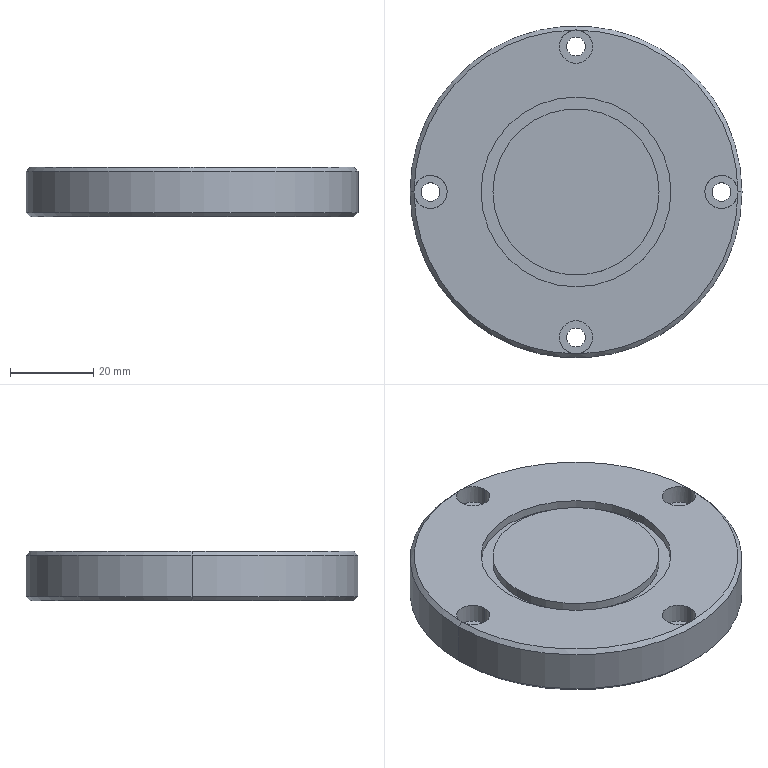Part | STEP file | TJ-DHQM-004-011 | 1 solid | 34 faces | box 79.9 x 79.9 x 12 mm | volume 57718 mm3 | cylinder 22 | plane 8 | cone 4 | commonest cylinder face diameters 4.5 x8 8 x8 40 x2 45.7 x2 79.9 x2
STEP:
#1=CARTESIAN_POINT('',(20.,0.,9.9));
#2=VERTEX_POINT('',#1);
#3=CARTESIAN_POINT('',(-20.,0.,9.9));
#4=VERTEX_POINT('',#3);
#5=CARTESIAN_POINT('',(0.,0.,9.9));
#6=DIRECTION('',(0.,0.,1.));
#7=DIRECTION('',(1.,0.,0.));
#8=AXIS2_PLACEMENT_3D('',#5,#6,#7);
#9=CIRCLE('',#8,20.);
#10=EDGE_CURVE('',#2,#4,#9,.T.);
#11=ORIENTED_EDGE('',*,*,#10,.T.);
#12=CARTESIAN_POINT('',(-20.,0.,12.));
#13=VERTEX_POINT('',#12);
#14=CARTESIAN_POINT('',(-20.,0.,9.9));
#15=DIRECTION('',(0.,0.,1.));
#16=VECTOR('',#15,1000.);
#17=LINE('',#14,#16);
#18=EDGE_CURVE('',#4,#13,#17,.T.);
#19=ORIENTED_EDGE('',*,*,#18,.T.);
#20=CARTESIAN_POINT('',(20.,0.,12.));
#21=VERTEX_POINT('',#20);
#22=CARTESIAN_POINT('',(0.,0.,12.));
#23=DIRECTION('',(0.,0.,1.));
#24=DIRECTION('',(1.,0.,0.));
#25=AXIS2_PLACEMENT_3D('',#22,#23,#24);
#26=CIRCLE('',#25,20.);
#27=EDGE_CURVE('',#21,#13,#26,.T.);
#28=ORIENTED_EDGE('',*,*,#27,.F.);
#29=CARTESIAN_POINT('',(20.,0.,9.9));
#30=DIRECTION('',(0.,0.,1.));
#31=VECTOR('',#30,1000.);
#32=LINE('',#29,#31);
#33=EDGE_CURVE('',#2,#21,#32,.T.);
#34=ORIENTED_EDGE('',*,*,#33,.F.);
#35=EDGE_LOOP('',(#11,#19,#28,#34));
#36=FACE_OUTER_BOUND('',#35,.T.);
#37=CARTESIAN_POINT('',(0.,0.,9.9));
#38=DIRECTION('',(0.,0.,1.));
#39=DIRECTION('',(1.,0.,0.));
#40=AXIS2_PLACEMENT_3D('',#37,#38,#39);
#41=CYLINDRICAL_SURFACE('',#40,20.);
#42=ADVANCED_FACE('',(#36),#41,.T.);
#43=CARTESIAN_POINT('',(-22.85,0.,9.9));
#44=VERTEX_POINT('',#43);
#45=CARTESIAN_POINT('',(22.85,0.,9.9));
#46=VERTEX_POINT('',#45);
#47=CARTESIAN_POINT('',(0.,0.,9.9));
#48=DIRECTION('',(0.,0.,1.));
#49=DIRECTION('',(1.,0.,0.));
#50=AXIS2_PLACEMENT_3D('',#47,#48,#49);
#51=CIRCLE('',#50,22.85);
#52=EDGE_CURVE('',#44,#46,#51,.T.);
#53=ORIENTED_EDGE('',*,*,#52,.F.);
#54=CARTESIAN_POINT('',(-22.85,0.,12.));
#55=VERTEX_POINT('',#54);
#56=CARTESIAN_POINT('',(-22.85,0.,9.9));
#57=DIRECTION('',(0.,0.,1.));
#58=VECTOR('',#57,1000.);
#59=LINE('',#56,#58);
#60=EDGE_CURVE('',#44,#55,#59,.T.);
#61=ORIENTED_EDGE('',*,*,#60,.T.);
#62=CARTESIAN_POINT('',(22.85,0.,12.));
#63=VERTEX_POINT('',#62);
#64=CARTESIAN_POINT('',(0.,0.,12.));
#65=DIRECTION('',(0.,0.,1.));
#66=DIRECTION('',(1.,0.,0.));
#67=AXIS2_PLACEMENT_3D('',#64,#65,#66);
#68=CIRCLE('',#67,22.85);
#69=EDGE_CURVE('',#55,#63,#68,.T.);
#70=ORIENTED_EDGE('',*,*,#69,.T.);
#71=CARTESIAN_POINT('',(22.85,0.,9.9));
#72=DIRECTION('',(0.,0.,1.));
#73=VECTOR('',#72,1000.);
#74=LINE('',#71,#73);
#75=EDGE_CURVE('',#46,#63,#74,.T.);
#76=ORIENTED_EDGE('',*,*,#75,.F.);
#77=EDGE_LOOP('',(#53,#61,#70,#76));
#78=FACE_OUTER_BOUND('',#77,.T.);
#79=CARTESIAN_POINT('',(0.,0.,9.9));
#80=DIRECTION('',(0.,0.,1.));
#81=DIRECTION('',(1.,0.,0.));
#82=AXIS2_PLACEMENT_3D('',#79,#80,#81);
#83=CYLINDRICAL_SURFACE('',#82,22.85);
#84=ADVANCED_FACE('',(#78),#83,.F.);
#85=CARTESIAN_POINT('',(-4.,35.,7.4));
#86=VERTEX_POINT('',#85);
#87=CARTESIAN_POINT('',(4.,35.,7.4));
#88=VERTEX_POINT('',#87);
#89=CARTESIAN_POINT('',(0.,35.,7.4));
#90=DIRECTION('',(0.,0.,1.));
#91=DIRECTION('',(1.,0.,0.));
#92=AXIS2_PLACEMENT_3D('',#89,#90,#91);
#93=CIRCLE('',#92,4.);
#94=EDGE_CURVE('',#86,#88,#93,.T.);
#95=ORIENTED_EDGE('',*,*,#94,.F.);
#96=CARTESIAN_POINT('',(-4.,35.,12.));
#97=VERTEX_POINT('',#96);
#98=CARTESIAN_POINT('',(-4.,35.,12.));
#99=DIRECTION('',(0.,0.,1.));
#100=VECTOR('',#99,1000.);
#101=LINE('',#98,#100);
#102=EDGE_CURVE('',#86,#97,#101,.T.);
#103=ORIENTED_EDGE('',*,*,#102,.T.);
#104=CARTESIAN_POINT('',(4.,35.,12.));
#105=VERTEX_POINT('',#104);
#106=CARTESIAN_POINT('',(0.,35.,12.));
#107=DIRECTION('',(0.,0.,1.));
#108=DIRECTION('',(1.,0.,0.));
#109=AXIS2_PLACEMENT_3D('',#106,#107,#108);
#110=CIRCLE('',#109,4.);
#111=EDGE_CURVE('',#97,#105,#110,.T.);
#112=ORIENTED_EDGE('',*,*,#111,.T.);
#113=CARTESIAN_POINT('',(4.,35.,12.));
#114=DIRECTION('',(0.,0.,1.));
#115=VECTOR('',#114,1000.);
#116=LINE('',#113,#115);
#117=EDGE_CURVE('',#88,#105,#116,.T.);
#118=ORIENTED_EDGE('',*,*,#117,.F.);
#119=EDGE_LOOP('',(#95,#103,#112,#118));
#120=FACE_OUTER_BOUND('',#119,.T.);
#121=CARTESIAN_POINT('',(0.,35.,12.));
#122=DIRECTION('',(0.,0.,1.));
#123=DIRECTION('',(1.,0.,0.));
#124=AXIS2_PLACEMENT_3D('',#121,#122,#123);
#125=CYLINDRICAL_SURFACE('',#124,4.);
#126=ADVANCED_FACE('',(#120),#125,.F.);
#127=CARTESIAN_POINT('',(-2.25,35.,0.));
#128=VERTEX_POINT('',#127);
#129=CARTESIAN_POINT('',(2.25,35.,0.));
#130=VERTEX_POINT('',#129);
#131=CARTESIAN_POINT('',(0.,35.,0.));
#132=DIRECTION('',(0.,0.,1.));
#133=DIRECTION('',(1.,0.,0.));
#134=AXIS2_PLACEMENT_3D('',#131,#132,#133);
#135=CIRCLE('',#134,2.25);
#136=EDGE_CURVE('',#128,#130,#135,.T.);
#137=ORIENTED_EDGE('',*,*,#136,.F.);
#138=CARTESIAN_POINT('',(-2.25,35.,7.4));
#139=VERTEX_POINT('',#138);
#140=CARTESIAN_POINT('',(-2.25,35.,12.));
#141=DIRECTION('',(0.,0.,1.));
#142=VECTOR('',#141,1000.);
#143=LINE('',#140,#142);
#144=EDGE_CURVE('',#128,#139,#143,.T.);
#145=ORIENTED_EDGE('',*,*,#144,.T.);
#146=CARTESIAN_POINT('',(2.25,35.,7.4));
#147=VERTEX_POINT('',#146);
#148=CARTESIAN_POINT('',(0.,35.,7.4));
#149=DIRECTION('',(0.,0.,1.));
#150=DIRECTION('',(1.,0.,0.));
#151=AXIS2_PLACEMENT_3D('',#148,#149,#150);
#152=CIRCLE('',#151,2.25);
#153=EDGE_CURVE('',#139,#147,#152,.T.);
#154=ORIENTED_EDGE('',*,*,#153,.T.);
#155=CARTESIAN_POINT('',(2.25,35.,12.));
#156=DIRECTION('',(0.,0.,1.));
#157=VECTOR('',#156,1000.);
#158=LINE('',#155,#157);
#159=EDGE_CURVE('',#130,#147,#158,.T.);
#160=ORIENTED_EDGE('',*,*,#159,.F.);
#161=EDGE_LOOP('',(#137,#145,#154,#160));
#162=FACE_OUTER_BOUND('',#161,.T.);
#163=CARTESIAN_POINT('',(0.,35.,12.));
#164=DIRECTION('',(0.,0.,1.));
#165=DIRECTION('',(1.,0.,0.));
#166=AXIS2_PLACEMENT_3D('',#163,#164,#165);
#167=CYLINDRICAL_SURFACE('',#166,2.25);
#168=ADVANCED_FACE('',(#162),#167,.F.);
#169=CARTESIAN_POINT('',(-39.,0.,7.4));
#170=VERTEX_POINT('',#169);
#171=CARTESIAN_POINT('',(-31.,0.,7.4));
#172=VERTEX_POINT('',#171);
#173=CARTESIAN_POINT('',(-35.,0.,7.4));
#174=DIRECTION('',(0.,0.,1.));
#175=DIRECTION('',(1.,0.,0.));
#176=AXIS2_PLACEMENT_3D('',#173,#174,#175);
#177=CIRCLE('',#176,4.);
#178=EDGE_CURVE('',#170,#172,#177,.T.);
#179=ORIENTED_EDGE('',*,*,#178,.F.);
#180=CARTESIAN_POINT('',(-39.,0.,11.95));
#181=VERTEX_POINT('',#180);
#182=CARTESIAN_POINT('',(-39.,0.,12.));
#183=DIRECTION('',(0.,0.,1.));
#184=VECTOR('',#183,1000.);
#185=LINE('',#182,#184);
#186=EDGE_CURVE('',#170,#181,#185,.T.);
#187=ORIENTED_EDGE('',*,*,#186,.T.);
#188=CARTESIAN_POINT('',(-38.944,-0.6651,12.));
#189=VERTEX_POINT('',#188);
#190=CARTESIAN_POINT('',(-39.,0.,11.95));
#191=CARTESIAN_POINT('',(-39.,-0.2216,11.95));
#192=CARTESIAN_POINT('',(-38.981,-0.4461,11.967));
#193=CARTESIAN_POINT('',(-38.944,-0.6651,12.));
#194=B_SPLINE_CURVE_WITH_KNOTS('',3,(#190,#191,#192,#193),.UNSPECIFIED.,.F.,.F.,(4,4),(0.0006695,0.001333),.UNSPECIFIED.);
#195=EDGE_CURVE('',#181,#189,#194,.T.);
#196=ORIENTED_EDGE('',*,*,#195,.T.);
#197=CARTESIAN_POINT('',(-31.,0.,12.));
#198=VERTEX_POINT('',#197);
#199=CARTESIAN_POINT('',(-35.,0.,12.));
#200=DIRECTION('',(0.,0.,1.));
#201=DIRECTION('',(1.,0.,0.));
#202=AXIS2_PLACEMENT_3D('',#199,#200,#201);
#203=CIRCLE('',#202,4.);
#204=EDGE_CURVE('',#189,#198,#203,.T.);
#205=ORIENTED_EDGE('',*,*,#204,.T.);
#206=CARTESIAN_POINT('',(-31.,0.,12.));
#207=DIRECTION('',(0.,0.,1.));
#208=VECTOR('',#207,1000.);
#209=LINE('',#206,#208);
#210=EDGE_CURVE('',#172,#198,#209,.T.);
#211=ORIENTED_EDGE('',*,*,#210,.F.);
#212=EDGE_LOOP('',(#179,#187,#196,#205,#211));
#213=FACE_OUTER_BOUND('',#212,.T.);
#214=CARTESIAN_POINT('',(-35.,0.,12.));
#215=DIRECTION('',(0.,0.,1.));
#216=DIRECTION('',(1.,0.,0.));
#217=AXIS2_PLACEMENT_3D('',#214,#215,#216);
#218=CYLINDRICAL_SURFACE('',#217,4.);
#219=ADVANCED_FACE('',(#213),#218,.F.);
#220=CARTESIAN_POINT('',(-37.25,0.,0.));
#221=VERTEX_POINT('',#220);
#222=CARTESIAN_POINT('',(-32.75,0.,0.));
#223=VERTEX_POINT('',#222);
#224=CARTESIAN_POINT('',(-35.,0.,0.));
#225=DIRECTION('',(0.,0.,1.));
#226=DIRECTION('',(1.,0.,0.));
#227=AXIS2_PLACEMENT_3D('',#224,#225,#226);
#228=CIRCLE('',#227,2.25);
#229=EDGE_CURVE('',#221,#223,#228,.T.);
#230=ORIENTED_EDGE('',*,*,#229,.F.);
#231=CARTESIAN_POINT('',(-37.25,0.,7.4));
#232=VERTEX_POINT('',#231);
#233=CARTESIAN_POINT('',(-37.25,0.,12.));
#234=DIRECTION('',(0.,0.,1.));
#235=VECTOR('',#234,1000.);
#236=LINE('',#233,#235);
#237=EDGE_CURVE('',#221,#232,#236,.T.);
#238=ORIENTED_EDGE('',*,*,#237,.T.);
#239=CARTESIAN_POINT('',(-32.75,0.,7.4));
#240=VERTEX_POINT('',#239);
#241=CARTESIAN_POINT('',(-35.,0.,7.4));
#242=DIRECTION('',(0.,0.,1.));
#243=DIRECTION('',(1.,0.,0.));
#244=AXIS2_PLACEMENT_3D('',#241,#242,#243);
#245=CIRCLE('',#244,2.25);
#246=EDGE_CURVE('',#232,#240,#245,.T.);
#247=ORIENTED_EDGE('',*,*,#246,.T.);
#248=CARTESIAN_POINT('',(-32.75,0.,12.));
#249=DIRECTION('',(0.,0.,1.));
#250=VECTOR('',#249,1000.);
#251=LINE('',#248,#250);
#252=EDGE_CURVE('',#223,#240,#251,.T.);
#253=ORIENTED_EDGE('',*,*,#252,.F.);
#254=EDGE_LOOP('',(#230,#238,#247,#253));
#255=FACE_OUTER_BOUND('',#254,.T.);
#256=CARTESIAN_POINT('',(-35.,0.,12.));
#257=DIRECTION('',(0.,0.,1.));
#258=DIRECTION('',(1.,0.,0.));
#259=AXIS2_PLACEMENT_3D('',#256,#257,#258);
#260=CYLINDRICAL_SURFACE('',#259,2.25);
#261=ADVANCED_FACE('',(#255),#260,.F.);
#262=CARTESIAN_POINT('',(-4.,-35.,7.4));
#263=VERTEX_POINT('',#262);
#264=CARTESIAN_POINT('',(4.,-35.,7.4));
#265=VERTEX_POINT('',#264);
#266=CARTESIAN_POINT('',(0.,-35.,7.4));
#267=DIRECTION('',(0.,0.,1.));
#268=DIRECTION('',(1.,0.,0.));
#269=AXIS2_PLACEMENT_3D('',#266,#267,#268);
#270=CIRCLE('',#269,4.);
#271=EDGE_CURVE('',#263,#265,#270,.T.);
#272=ORIENTED_EDGE('',*,*,#271,.F.);
#273=CARTESIAN_POINT('',(-4.,-35.,12.));
#274=VERTEX_POINT('',#273);
#275=CARTESIAN_POINT('',(-4.,-35.,12.));
#276=DIRECTION('',(0.,0.,1.));
#277=VECTOR('',#276,1000.);
#278=LINE('',#275,#277);
#279=EDGE_CURVE('',#263,#274,#278,.T.);
#280=ORIENTED_EDGE('',*,*,#279,.T.);
#281=CARTESIAN_POINT('',(-0.6651,-38.944,12.));
#282=VERTEX_POINT('',#281);
#283=CARTESIAN_POINT('',(0.,-35.,12.));
#284=DIRECTION('',(0.,0.,1.));
#285=DIRECTION('',(1.,0.,0.));
#286=AXIS2_PLACEMENT_3D('',#283,#284,#285);
#287=CIRCLE('',#286,4.);
#288=EDGE_CURVE('',#274,#282,#287,.T.);
#289=ORIENTED_EDGE('',*,*,#288,.T.);
#290=CARTESIAN_POINT('',(0.6651,-38.944,12.));
#291=VERTEX_POINT('',#290);
#292=CARTESIAN_POINT('',(-0.6651,-38.944,12.));
#293=CARTESIAN_POINT('',(-0.4455,-38.981,11.967));
#294=CARTESIAN_POINT('',(-0.2245,-39.,11.95));
#295=CARTESIAN_POINT('',(0.2202,-39.,11.95));
#296=CARTESIAN_POINT('',(0.4454,-38.981,11.967));
#297=CARTESIAN_POINT('',(0.6651,-38.944,12.));
#298=B_SPLINE_CURVE_WITH_KNOTS('',3,(#292,#293,#294,#295,#296,#297),.UNSPECIFIED.,.F.,.F.,(4,2,4),(0.000001333,0.0006674,0.001333),.UNSPECIFIED.);
#299=EDGE_CURVE('',#282,#291,#298,.T.);
#300=ORIENTED_EDGE('',*,*,#299,.T.);
#301=CARTESIAN_POINT('',(4.,-35.,12.));
#302=VERTEX_POINT('',#301);
#303=CARTESIAN_POINT('',(0.,-35.,12.));
#304=DIRECTION('',(0.,0.,1.));
#305=DIRECTION('',(1.,0.,0.));
#306=AXIS2_PLACEMENT_3D('',#303,#304,#305);
#307=CIRCLE('',#306,4.);
#308=EDGE_CURVE('',#291,#302,#307,.T.);
#309=ORIENTED_EDGE('',*,*,#308,.T.);
#310=CARTESIAN_POINT('',(4.,-35.,12.));
#311=DIRECTION('',(0.,0.,1.));
#312=VECTOR('',#311,1000.);
#313=LINE('',#310,#312);
#314=EDGE_CURVE('',#265,#302,#313,.T.);
#315=ORIENTED_EDGE('',*,*,#314,.F.);
#316=EDGE_LOOP('',(#272,#280,#289,#300,#309,#315));
#317=FACE_OUTER_BOUND('',#316,.T.);
#318=CARTESIAN_POINT('',(0.,-35.,12.));
#319=DIRECTION('',(0.,0.,1.));
#320=DIRECTION('',(1.,0.,0.));
#321=AXIS2_PLACEMENT_3D('',#318,#319,#320);
#322=CYLINDRICAL_SURFACE('',#321,4.);
#323=ADVANCED_FACE('',(#317),#322,.F.);
#324=CARTESIAN_POINT('',(-2.25,-35.,0.));
#325=VERTEX_POINT('',#324);
#326=CARTESIAN_POINT('',(2.25,-35.,0.));
#327=VERTEX_POINT('',#326);
#328=CARTESIAN_POINT('',(0.,-35.,0.));
#329=DIRECTION('',(0.,0.,1.));
#330=DIRECTION('',(1.,0.,0.));
#331=AXIS2_PLACEMENT_3D('',#328,#329,#330);
#332=CIRCLE('',#331,2.25);
#333=EDGE_CURVE('',#325,#327,#332,.T.);
#334=ORIENTED_EDGE('',*,*,#333,.F.);
#335=CARTESIAN_POINT('',(-2.25,-35.,7.4));
#336=VERTEX_POINT('',#335);
#337=CARTESIAN_POINT('',(-2.25,-35.,12.));
#338=DIRECTION('',(0.,0.,1.));
#339=VECTOR('',#338,1000.);
#340=LINE('',#337,#339);
#341=EDGE_CURVE('',#325,#336,#340,.T.);
#342=ORIENTED_EDGE('',*,*,#341,.T.);
#343=CARTESIAN_POINT('',(2.25,-35.,7.4));
#344=VERTEX_POINT('',#343);
#345=CARTESIAN_POINT('',(0.,-35.,7.4));
#346=DIRECTION('',(0.,0.,1.));
#347=DIRECTION('',(1.,0.,0.));
#348=AXIS2_PLACEMENT_3D('',#345,#346,#347);
#349=CIRCLE('',#348,2.25);
#350=EDGE_CURVE('',#336,#344,#349,.T.);
#351=ORIENTED_EDGE('',*,*,#350,.T.);
#352=CARTESIAN_POINT('',(2.25,-35.,12.));
#353=DIRECTION('',(0.,0.,1.));
#354=VECTOR('',#353,1000.);
#355=LINE('',#352,#354);
#356=EDGE_CURVE('',#327,#344,#355,.T.);
#357=ORIENTED_EDGE('',*,*,#356,.F.);
#358=EDGE_LOOP('',(#334,#342,#351,#357));
#359=FACE_OUTER_BOUND('',#358,.T.);
#360=CARTESIAN_POINT('',(0.,-35.,12.));
#361=DIRECTION('',(0.,0.,1.));
#362=DIRECTION('',(1.,0.,0.));
#363=AXIS2_PLACEMENT_3D('',#360,#361,#362);
#364=CYLINDRICAL_SURFACE('',#363,2.25);
#365=ADVANCED_FACE('',(#359),#364,.F.);
#366=CARTESIAN_POINT('',(31.,0.,7.4));
#367=VERTEX_POINT('',#366);
#368=CARTESIAN_POINT('',(39.,0.,7.4));
#369=VERTEX_POINT('',#368);
#370=CARTESIAN_POINT('',(35.,0.,7.4));
#371=DIRECTION('',(0.,0.,1.));
#372=DIRECTION('',(1.,0.,0.));
#373=AXIS2_PLACEMENT_3D('',#370,#371,#372);
#374=CIRCLE('',#373,4.);
#375=EDGE_CURVE('',#367,#369,#374,.T.);
#376=ORIENTED_EDGE('',*,*,#375,.F.);
#377=CARTESIAN_POINT('',(31.,0.,12.));
#378=VERTEX_POINT('',#377);
#379=CARTESIAN_POINT('',(31.,0.,12.));
#380=DIRECTION('',(0.,0.,1.));
#381=VECTOR('',#380,1000.);
#382=LINE('',#379,#381);
#383=EDGE_CURVE('',#367,#378,#382,.T.);
#384=ORIENTED_EDGE('',*,*,#383,.T.);
#385=CARTESIAN_POINT('',(38.944,-0.6651,12.));
#386=VERTEX_POINT('',#385);
#387=CARTESIAN_POINT('',(35.,0.,12.));
#388=DIRECTION('',(0.,0.,1.));
#389=DIRECTION('',(1.,0.,0.));
#390=AXIS2_PLACEMENT_3D('',#387,#388,#389);
#391=CIRCLE('',#390,4.);
#392=EDGE_CURVE('',#378,#386,#391,.T.);
#393=ORIENTED_EDGE('',*,*,#392,.T.);
#394=CARTESIAN_POINT('',(39.,0.,11.95));
#395=VERTEX_POINT('',#394);
#396=CARTESIAN_POINT('',(38.944,-0.6651,12.));
#397=CARTESIAN_POINT('',(38.981,-0.4448,11.967));
#398=CARTESIAN_POINT('',(39.,-0.2231,11.95));
#399=CARTESIAN_POINT('',(39.,0.,11.95));
#400=B_SPLINE_CURVE_WITH_KNOTS('',3,(#396,#397,#398,#399),.UNSPECIFIED.,.F.,.F.,(4,4),(0.000001333,0.0006695),.UNSPECIFIED.);
#401=EDGE_CURVE('',#386,#395,#400,.T.);
#402=ORIENTED_EDGE('',*,*,#401,.T.);
#403=CARTESIAN_POINT('',(39.,0.,12.));
#404=DIRECTION('',(0.,0.,1.));
#405=VECTOR('',#404,1000.);
#406=LINE('',#403,#405);
#407=EDGE_CURVE('',#369,#395,#406,.T.);
#408=ORIENTED_EDGE('',*,*,#407,.F.);
#409=EDGE_LOOP('',(#376,#384,#393,#402,#408));
#410=FACE_OUTER_BOUND('',#409,.T.);
#411=CARTESIAN_POINT('',(35.,0.,12.));
#412=DIRECTION('',(0.,0.,1.));
#413=DIRECTION('',(1.,0.,0.));
#414=AXIS2_PLACEMENT_3D('',#411,#412,#413);
#415=CYLINDRICAL_SURFACE('',#414,4.);
#416=ADVANCED_FACE('',(#410),#415,.F.);
#417=CARTESIAN_POINT('',(32.75,0.,0.));
#418=VERTEX_POINT('',#417);
#419=CARTESIAN_POINT('',(37.25,0.,0.));
#420=VERTEX_POINT('',#419);
#421=CARTESIAN_POINT('',(35.,0.,0.));
#422=DIRECTION('',(0.,0.,1.));
#423=DIRECTION('',(1.,0.,0.));
#424=AXIS2_PLACEMENT_3D('',#421,#422,#423);
#425=CIRCLE('',#424,2.25);
#426=EDGE_CURVE('',#418,#420,#425,.T.);
#427=ORIENTED_EDGE('',*,*,#426,.F.);
#428=CARTESIAN_POINT('',(32.75,0.,7.4));
#429=VERTEX_POINT('',#428);
#430=CARTESIAN_POINT('',(32.75,0.,12.));
#431=DIRECTION('',(0.,0.,1.));
#432=VECTOR('',#431,1000.);
#433=LINE('',#430,#432);
#434=EDGE_CURVE('',#418,#429,#433,.T.);
#435=ORIENTED_EDGE('',*,*,#434,.T.);
#436=CARTESIAN_POINT('',(37.25,0.,7.4));
#437=VERTEX_POINT('',#436);
#438=CARTESIAN_POINT('',(35.,0.,7.4));
#439=DIRECTION('',(0.,0.,1.));
#440=DIRECTION('',(1.,0.,0.));
#441=AXIS2_PLACEMENT_3D('',#438,#439,#440);
#442=CIRCLE('',#441,2.25);
#443=EDGE_CURVE('',#429,#437,#442,.T.);
#444=ORIENTED_EDGE('',*,*,#443,.T.);
#445=CARTESIAN_POINT('',(37.25,0.,12.));
#446=DIRECTION('',(0.,0.,1.));
#447=VECTOR('',#446,1000.);
#448=LINE('',#445,#447);
#449=EDGE_CURVE('',#420,#437,#448,.T.);
#450=ORIENTED_EDGE('',*,*,#449,.F.);
#451=EDGE_LOOP('',(#427,#435,#444,#450));
#452=FACE_OUTER_BOUND('',#451,.T.);
#453=CARTESIAN_POINT('',(35.,0.,12.));
#454=DIRECTION('',(0.,0.,1.));
#455=DIRECTION('',(1.,0.,0.));
#456=AXIS2_PLACEMENT_3D('',#453,#454,#455);
#457=CYLINDRICAL_SURFACE('',#456,2.25);
#458=ADVANCED_FACE('',(#452),#457,.F.);
#459=CARTESIAN_POINT('',(38.944,0.6651,12.));
#460=VERTEX_POINT('',#459);
#461=CARTESIAN_POINT('',(39.,0.,11.95));
#462=CARTESIAN_POINT('',(39.,0.2216,11.95));
#463=CARTESIAN_POINT('',(38.981,0.4461,11.967));
#464=CARTESIAN_POINT('',(38.944,0.6651,12.));
#465=B_SPLINE_CURVE_WITH_KNOTS('',3,(#461,#462,#463,#464),.UNSPECIFIED.,.F.,.F.,(4,4),(0.0006695,0.001333),.UNSPECIFIED.);
#466=EDGE_CURVE('',#395,#460,#465,.T.);
#467=ORIENTED_EDGE('',*,*,#466,.F.);
#468=CARTESIAN_POINT('',(39.95,0.,11.));
#469=VERTEX_POINT('',#468);
#470=CARTESIAN_POINT('',(38.95,0.,12.));
#471=DIRECTION('',(0.7071,0.,-0.7071));
#472=VECTOR('',#471,1000.);
#473=LINE('',#470,#472);
#474=EDGE_CURVE('',#395,#469,#473,.T.);
#475=ORIENTED_EDGE('',*,*,#474,.T.);
#476=CARTESIAN_POINT('',(-39.95,0.,11.));
#477=VERTEX_POINT('',#476);
#478=CARTESIAN_POINT('',(0.,0.,11.));
#479=DIRECTION('',(0.,0.,-1.));
#480=DIRECTION('',(1.,0.,0.));
#481=AXIS2_PLACEMENT_3D('',#478,#479,#480);
#482=CIRCLE('',#481,39.95);
#483=EDGE_CURVE('',#477,#469,#482,.T.);
#484=ORIENTED_EDGE('',*,*,#483,.F.);
#485=CARTESIAN_POINT('',(-38.95,0.,12.));
#486=DIRECTION('',(-0.7071,0.,-0.7071));
#487=VECTOR('',#486,1000.);
#488=LINE('',#485,#487);
#489=EDGE_CURVE('',#181,#477,#488,.T.);
#490=ORIENTED_EDGE('',*,*,#489,.F.);
#491=CARTESIAN_POINT('',(-38.944,0.6651,12.));
#492=VERTEX_POINT('',#491);
#493=CARTESIAN_POINT('',(-38.944,0.6651,12.));
#494=CARTESIAN_POINT('',(-38.981,0.4448,11.967));
#495=CARTESIAN_POINT('',(-39.,0.2231,11.95));
#496=CARTESIAN_POINT('',(-39.,0.,11.95));
#497=B_SPLINE_CURVE_WITH_KNOTS('',3,(#493,#494,#495,#496),.UNSPECIFIED.,.F.,.F.,(4,4),(0.000001333,0.0006695),.UNSPECIFIED.);
#498=EDGE_CURVE('',#492,#181,#497,.T.);
#499=ORIENTED_EDGE('',*,*,#498,.F.);
#500=CARTESIAN_POINT('',(-0.6651,38.944,12.));
#501=VERTEX_POINT('',#500);
#502=CARTESIAN_POINT('',(0.,0.,12.));
#503=DIRECTION('',(0.,0.,1.));
#504=DIRECTION('',(1.,0.,0.));
#505=AXIS2_PLACEMENT_3D('',#502,#503,#504);
#506=CIRCLE('',#505,38.95);
#507=EDGE_CURVE('',#501,#492,#506,.T.);
#508=ORIENTED_EDGE('',*,*,#507,.F.);
#509=CARTESIAN_POINT('',(0.6651,38.944,12.));
#510=VERTEX_POINT('',#509);
#511=CARTESIAN_POINT('',(0.6651,38.944,12.));
#512=CARTESIAN_POINT('',(0.4455,38.981,11.967));
#513=CARTESIAN_POINT('',(0.2245,39.,11.95));
#514=CARTESIAN_POINT('',(-0.2202,39.,11.95));
#515=CARTESIAN_POINT('',(-0.4454,38.981,11.967));
#516=CARTESIAN_POINT('',(-0.6651,38.944,12.));
#517=B_SPLINE_CURVE_WITH_KNOTS('',3,(#511,#512,#513,#514,#515,#516),.UNSPECIFIED.,.F.,.F.,(4,2,4),(0.000001333,0.0006674,0.001333),.UNSPECIFIED.);
#518=EDGE_CURVE('',#510,#501,#517,.T.);
#519=ORIENTED_EDGE('',*,*,#518,.F.);
#520=CARTESIAN_POINT('',(0.,0.,12.));
#521=DIRECTION('',(0.,0.,1.));
#522=DIRECTION('',(1.,0.,0.));
#523=AXIS2_PLACEMENT_3D('',#520,#521,#522);
#524=CIRCLE('',#523,38.95);
#525=EDGE_CURVE('',#460,#510,#524,.T.);
#526=ORIENTED_EDGE('',*,*,#525,.F.);
#527=EDGE_LOOP('',(#467,#475,#484,#490,#499,#508,#519,#526));
#528=FACE_OUTER_BOUND('',#527,.T.);
#529=CARTESIAN_POINT('',(0.,0.,12.));
#530=DIRECTION('',(0.,0.,-1.));
#531=DIRECTION('',(-1.,0.,0.));
#532=AXIS2_PLACEMENT_3D('',#529,#530,#531);
#533=CONICAL_SURFACE('',#532,38.95,0.7854);
#534=ADVANCED_FACE('',(#528),#533,.T.);
#535=CARTESIAN_POINT('',(-38.95,0.,0.));
#536=VERTEX_POINT('',#535);
#537=CARTESIAN_POINT('',(38.95,0.,0.));
#538=VERTEX_POINT('',#537);
#539=CARTESIAN_POINT('',(0.,0.,0.));
#540=DIRECTION('',(0.,0.,-1.));
#541=DIRECTION('',(1.,0.,0.));
#542=AXIS2_PLACEMENT_3D('',#539,#540,#541);
#543=CIRCLE('',#542,38.95);
#544=EDGE_CURVE('',#536,#538,#543,.T.);
#545=ORIENTED_EDGE('',*,*,#544,.F.);
#546=CARTESIAN_POINT('',(-39.95,0.,1.));
#547=VERTEX_POINT('',#546);
#548=CARTESIAN_POINT('',(-39.95,0.,1.));
#549=DIRECTION('',(-0.7071,0.,0.7071));
#550=VECTOR('',#549,1000.);
#551=LINE('',#548,#550);
#552=EDGE_CURVE('',#536,#547,#551,.T.);
#553=ORIENTED_EDGE('',*,*,#552,.T.);
#554=CARTESIAN_POINT('',(39.95,0.,1.));
#555=VERTEX_POINT('',#554);
#556=CARTESIAN_POINT('',(0.,0.,1.));
#557=DIRECTION('',(0.,0.,1.));
#558=DIRECTION('',(1.,0.,0.));
#559=AXIS2_PLACEMENT_3D('',#556,#557,#558);
#560=CIRCLE('',#559,39.95);
#561=EDGE_CURVE('',#555,#547,#560,.T.);
#562=ORIENTED_EDGE('',*,*,#561,.F.);
#563=CARTESIAN_POINT('',(39.95,0.,1.));
#564=DIRECTION('',(0.7071,0.,0.7071));
#565=VECTOR('',#564,1000.);
#566=LINE('',#563,#565);
#567=EDGE_CURVE('',#538,#555,#566,.T.);
#568=ORIENTED_EDGE('',*,*,#567,.F.);
#569=EDGE_LOOP('',(#545,#553,#562,#568));
#570=FACE_OUTER_BOUND('',#569,.T.);
#571=CARTESIAN_POINT('',(0.,0.,1.));
#572=DIRECTION('',(0.,0.,1.));
#573=DIRECTION('',(1.,0.,0.));
#574=AXIS2_PLACEMENT_3D('',#571,#572,#573);
#575=CONICAL_SURFACE('',#574,39.95,0.7854);
#576=ADVANCED_FACE('',(#570),#575,.T.);
#577=ORIENTED_EDGE('',*,*,#483,.T.);
#578=CARTESIAN_POINT('',(39.95,0.,12.));
#579=DIRECTION('',(0.,0.,-1.));
#580=VECTOR('',#579,1000.);
#581=LINE('',#578,#580);
#582=EDGE_CURVE('',#469,#555,#581,.T.);
#583=ORIENTED_EDGE('',*,*,#582,.T.);
#584=ORIENTED_EDGE('',*,*,#561,.T.);
#585=CARTESIAN_POINT('',(-39.95,0.,12.));
#586=DIRECTION('',(0.,0.,-1.));
#587=VECTOR('',#586,1000.);
#588=LINE('',#585,#587);
#589=EDGE_CURVE('',#477,#547,#588,.T.);
#590=ORIENTED_EDGE('',*,*,#589,.F.);
#591=EDGE_LOOP('',(#577,#583,#584,#590));
#592=FACE_OUTER_BOUND('',#591,.T.);
#593=CARTESIAN_POINT('',(0.,0.,12.));
#594=DIRECTION('',(0.,0.,-1.));
#595=DIRECTION('',(-1.,0.,0.));
#596=AXIS2_PLACEMENT_3D('',#593,#594,#595);
#597=CYLINDRICAL_SURFACE('',#596,39.95);
#598=ADVANCED_FACE('',(#592),#597,.T.);
#599=ORIENTED_EDGE('',*,*,#582,.F.);
#600=CARTESIAN_POINT('',(0.,0.,11.));
#601=DIRECTION('',(0.,0.,-1.));
#602=DIRECTION('',(1.,0.,0.));
#603=AXIS2_PLACEMENT_3D('',#600,#601,#602);
#604=CIRCLE('',#603,39.95);
#605=EDGE_CURVE('',#469,#477,#604,.T.);
#606=ORIENTED_EDGE('',*,*,#605,.T.);
#607=ORIENTED_EDGE('',*,*,#589,.T.);
#608=CARTESIAN_POINT('',(0.,0.,1.));
#609=DIRECTION('',(0.,0.,1.));
#610=DIRECTION('',(1.,0.,0.));
#611=AXIS2_PLACEMENT_3D('',#608,#609,#610);
#612=CIRCLE('',#611,39.95);
#613=EDGE_CURVE('',#547,#555,#612,.T.);
#614=ORIENTED_EDGE('',*,*,#613,.T.);
#615=EDGE_LOOP('',(#599,#606,#607,#614));
#616=FACE_OUTER_BOUND('',#615,.T.);
#617=CARTESIAN_POINT('',(0.,0.,12.));
#618=DIRECTION('',(0.,0.,-1.));
#619=DIRECTION('',(-1.,0.,0.));
#620=AXIS2_PLACEMENT_3D('',#617,#618,#619);
#621=CYLINDRICAL_SURFACE('',#620,39.95);
#622=ADVANCED_FACE('',(#616),#621,.T.);
#623=CARTESIAN_POINT('',(0.,0.,12.));
#624=DIRECTION('',(0.,0.,1.));
#625=DIRECTION('',(1.,0.,0.));
#626=AXIS2_PLACEMENT_3D('',#623,#624,#625);
#627=CIRCLE('',#626,22.85);
#628=EDGE_CURVE('',#63,#55,#627,.T.);
#629=ORIENTED_EDGE('',*,*,#628,.F.);
#630=ORIENTED_EDGE('',*,*,#69,.F.);
#631=EDGE_LOOP('',(#629,#630));
#632=FACE_BOUND('',#631,.T.);
#633=CARTESIAN_POINT('',(0.,35.,12.));
#634=DIRECTION('',(0.,0.,1.));
#635=DIRECTION('',(1.,0.,0.));
#636=AXIS2_PLACEMENT_3D('',#633,#634,#635);
#637=CIRCLE('',#636,4.);
#638=EDGE_CURVE('',#501,#97,#637,.T.);
#639=ORIENTED_EDGE('',*,*,#638,.F.);
#640=ORIENTED_EDGE('',*,*,#507,.T.);
#641=CARTESIAN_POINT('',(-35.,0.,12.));
#642=DIRECTION('',(0.,0.,1.));
#643=DIRECTION('',(1.,0.,0.));
#644=AXIS2_PLACEMENT_3D('',#641,#642,#643);
#645=CIRCLE('',#644,4.);
#646=EDGE_CURVE('',#198,#492,#645,.T.);
#647=ORIENTED_EDGE('',*,*,#646,.F.);
#648=ORIENTED_EDGE('',*,*,#204,.F.);
#649=CARTESIAN_POINT('',(0.,0.,12.));
#650=DIRECTION('',(0.,0.,1.));
#651=DIRECTION('',(1.,0.,0.));
#652=AXIS2_PLACEMENT_3D('',#649,#650,#651);
#653=CIRCLE('',#652,38.95);
#654=EDGE_CURVE('',#189,#282,#653,.T.);
#655=ORIENTED_EDGE('',*,*,#654,.T.);
#656=ORIENTED_EDGE('',*,*,#288,.F.);
#657=CARTESIAN_POINT('',(0.,-35.,12.));
#658=DIRECTION('',(0.,0.,1.));
#659=DIRECTION('',(1.,0.,0.));
#660=AXIS2_PLACEMENT_3D('',#657,#658,#659);
#661=CIRCLE('',#660,4.);
#662=EDGE_CURVE('',#302,#274,#661,.T.);
#663=ORIENTED_EDGE('',*,*,#662,.F.);
#664=ORIENTED_EDGE('',*,*,#308,.F.);
#665=CARTESIAN_POINT('',(0.,0.,12.));
#666=DIRECTION('',(0.,0.,1.));
#667=DIRECTION('',(1.,0.,0.));
#668=AXIS2_PLACEMENT_3D('',#665,#666,#667);
#669=CIRCLE('',#668,38.95);
#670=EDGE_CURVE('',#291,#386,#669,.T.);
#671=ORIENTED_EDGE('',*,*,#670,.T.);
#672=ORIENTED_EDGE('',*,*,#392,.F.);
#673=CARTESIAN_POINT('',(35.,0.,12.));
#674=DIRECTION('',(0.,0.,1.));
#675=DIRECTION('',(1.,0.,0.));
#676=AXIS2_PLACEMENT_3D('',#673,#674,#675);
#677=CIRCLE('',#676,4.);
#678=EDGE_CURVE('',#460,#378,#677,.T.);
#679=ORIENTED_EDGE('',*,*,#678,.F.);
#680=ORIENTED_EDGE('',*,*,#525,.T.);
#681=CARTESIAN_POINT('',(0.,35.,12.));
#682=DIRECTION('',(0.,0.,1.));
#683=DIRECTION('',(1.,0.,0.));
#684=AXIS2_PLACEMENT_3D('',#681,#682,#683);
#685=CIRCLE('',#684,4.);
#686=EDGE_CURVE('',#105,#510,#685,.T.);
#687=ORIENTED_EDGE('',*,*,#686,.F.);
#688=ORIENTED_EDGE('',*,*,#111,.F.);
#689=EDGE_LOOP('',(#639,#640,#647,#648,#655,#656,#663,#664,#671,#672,#679,#680,#687,#688));
#690=FACE_OUTER_BOUND('',#689,.T.);
#691=CARTESIAN_POINT('',(0.,0.,12.));
#692=DIRECTION('',(0.,0.,1.));
#693=DIRECTION('',(1.,0.,0.));
#694=AXIS2_PLACEMENT_3D('',#691,#692,#693);
#695=PLANE('',#694);
#696=ADVANCED_FACE('',(#632,#690),#695,.T.);
#697=CARTESIAN_POINT('',(0.,35.,0.));
#698=DIRECTION('',(0.,0.,1.));
#699=DIRECTION('',(1.,0.,0.));
#700=AXIS2_PLACEMENT_3D('',#697,#698,#699);
#701=CIRCLE('',#700,2.25);
#702=EDGE_CURVE('',#130,#128,#701,.T.);
#703=ORIENTED_EDGE('',*,*,#702,.T.);
#704=ORIENTED_EDGE('',*,*,#136,.T.);
#705=EDGE_LOOP('',(#703,#704));
#706=FACE_BOUND('',#705,.T.);
#707=CARTESIAN_POINT('',(-35.,0.,0.));
#708=DIRECTION('',(0.,0.,1.));
#709=DIRECTION('',(1.,0.,0.));
#710=AXIS2_PLACEMENT_3D('',#707,#708,#709);
#711=CIRCLE('',#710,2.25);
#712=EDGE_CURVE('',#223,#221,#711,.T.);
#713=ORIENTED_EDGE('',*,*,#712,.T.);
#714=ORIENTED_EDGE('',*,*,#229,.T.);
#715=EDGE_LOOP('',(#713,#714));
#716=FACE_BOUND('',#715,.T.);
#717=CARTESIAN_POINT('',(0.,-35.,0.));
#718=DIRECTION('',(0.,0.,1.));
#719=DIRECTION('',(1.,0.,0.));
#720=AXIS2_PLACEMENT_3D('',#717,#718,#719);
#721=CIRCLE('',#720,2.25);
#722=EDGE_CURVE('',#327,#325,#721,.T.);
#723=ORIENTED_EDGE('',*,*,#722,.T.);
#724=ORIENTED_EDGE('',*,*,#333,.T.);
#725=EDGE_LOOP('',(#723,#724));
#726=FACE_BOUND('',#725,.T.);
#727=CARTESIAN_POINT('',(35.,0.,0.));
#728=DIRECTION('',(0.,0.,1.));
#729=DIRECTION('',(1.,0.,0.));
#730=AXIS2_PLACEMENT_3D('',#727,#728,#729);
#731=CIRCLE('',#730,2.25);
#732=EDGE_CURVE('',#420,#418,#731,.T.);
#733=ORIENTED_EDGE('',*,*,#732,.T.);
#734=ORIENTED_EDGE('',*,*,#426,.T.);
#735=EDGE_LOOP('',(#733,#734));
#736=FACE_BOUND('',#735,.T.);
#737=CARTESIAN_POINT('',(0.,0.,0.));
#738=DIRECTION('',(0.,0.,-1.));
#739=DIRECTION('',(1.,0.,0.));
#740=AXIS2_PLACEMENT_3D('',#737,#738,#739);
#741=CIRCLE('',#740,38.95);
#742=EDGE_CURVE('',#538,#536,#741,.T.);
#743=ORIENTED_EDGE('',*,*,#742,.T.);
#744=ORIENTED_EDGE('',*,*,#544,.T.);
#745=EDGE_LOOP('',(#743,#744));
#746=FACE_OUTER_BOUND('',#745,.T.);
#747=CARTESIAN_POINT('',(0.,0.,0.));
#748=DIRECTION('',(0.,0.,1.));
#749=DIRECTION('',(1.,0.,0.));
#750=AXIS2_PLACEMENT_3D('',#747,#748,#749);
#751=PLANE('',#750);
#752=ADVANCED_FACE('',(#706,#716,#726,#736,#746),#751,.F.);
#753=ORIENTED_EDGE('',*,*,#552,.F.);
#754=ORIENTED_EDGE('',*,*,#742,.F.);
#755=ORIENTED_EDGE('',*,*,#567,.T.);
#756=ORIENTED_EDGE('',*,*,#613,.F.);
#757=EDGE_LOOP('',(#753,#754,#755,#756));
#758=FACE_OUTER_BOUND('',#757,.T.);
#759=CARTESIAN_POINT('',(0.,0.,1.));
#760=DIRECTION('',(0.,0.,1.));
#761=DIRECTION('',(1.,0.,0.));
#762=AXIS2_PLACEMENT_3D('',#759,#760,#761);
#763=CONICAL_SURFACE('',#762,39.95,0.7854);
#764=ADVANCED_FACE('',(#758),#763,.T.);
#765=ORIENTED_EDGE('',*,*,#474,.F.);
#766=ORIENTED_EDGE('',*,*,#401,.F.);
#767=ORIENTED_EDGE('',*,*,#670,.F.);
#768=ORIENTED_EDGE('',*,*,#299,.F.);
#769=ORIENTED_EDGE('',*,*,#654,.F.);
#770=ORIENTED_EDGE('',*,*,#195,.F.);
#771=ORIENTED_EDGE('',*,*,#489,.T.);
#772=ORIENTED_EDGE('',*,*,#605,.F.);
#773=EDGE_LOOP('',(#765,#766,#767,#768,#769,#770,#771,#772));
#774=FACE_OUTER_BOUND('',#773,.T.);
#775=CARTESIAN_POINT('',(0.,0.,12.));
#776=DIRECTION('',(0.,0.,-1.));
#777=DIRECTION('',(-1.,0.,0.));
#778=AXIS2_PLACEMENT_3D('',#775,#776,#777);
#779=CONICAL_SURFACE('',#778,38.95,0.7854);
#780=ADVANCED_FACE('',(#774),#779,.T.);
#781=ORIENTED_EDGE('',*,*,#434,.F.);
#782=ORIENTED_EDGE('',*,*,#732,.F.);
#783=ORIENTED_EDGE('',*,*,#449,.T.);
#784=CARTESIAN_POINT('',(35.,0.,7.4));
#785=DIRECTION('',(0.,0.,1.));
#786=DIRECTION('',(1.,0.,0.));
#787=AXIS2_PLACEMENT_3D('',#784,#785,#786);
#788=CIRCLE('',#787,2.25);
#789=EDGE_CURVE('',#437,#429,#788,.T.);
#790=ORIENTED_EDGE('',*,*,#789,.T.);
#791=EDGE_LOOP('',(#781,#782,#783,#790));
#792=FACE_OUTER_BOUND('',#791,.T.);
#793=CARTESIAN_POINT('',(35.,0.,12.));
#794=DIRECTION('',(0.,0.,1.));
#795=DIRECTION('',(1.,0.,0.));
#796=AXIS2_PLACEMENT_3D('',#793,#794,#795);
#797=CYLINDRICAL_SURFACE('',#796,2.25);
#798=ADVANCED_FACE('',(#792),#797,.F.);
#799=ORIENTED_EDGE('',*,*,#789,.F.);
#800=ORIENTED_EDGE('',*,*,#443,.F.);
#801=EDGE_LOOP('',(#799,#800));
#802=FACE_BOUND('',#801,.T.);
#803=CARTESIAN_POINT('',(35.,0.,7.4));
#804=DIRECTION('',(0.,0.,1.));
#805=DIRECTION('',(1.,0.,0.));
#806=AXIS2_PLACEMENT_3D('',#803,#804,#805);
#807=CIRCLE('',#806,4.);
#808=EDGE_CURVE('',#369,#367,#807,.T.);
#809=ORIENTED_EDGE('',*,*,#808,.T.);
#810=ORIENTED_EDGE('',*,*,#375,.T.);
#811=EDGE_LOOP('',(#809,#810));
#812=FACE_OUTER_BOUND('',#811,.T.);
#813=CARTESIAN_POINT('',(37.25,0.,7.4));
#814=DIRECTION('',(0.,0.,-1.));
#815=DIRECTION('',(-1.,0.,0.));
#816=AXIS2_PLACEMENT_3D('',#813,#814,#815);
#817=PLANE('',#816);
#818=ADVANCED_FACE('',(#802,#812),#817,.F.);
#819=ORIENTED_EDGE('',*,*,#383,.F.);
#820=ORIENTED_EDGE('',*,*,#808,.F.);
#821=ORIENTED_EDGE('',*,*,#407,.T.);
#822=ORIENTED_EDGE('',*,*,#466,.T.);
#823=ORIENTED_EDGE('',*,*,#678,.T.);
#824=EDGE_LOOP('',(#819,#820,#821,#822,#823));
#825=FACE_OUTER_BOUND('',#824,.T.);
#826=CARTESIAN_POINT('',(35.,0.,12.));
#827=DIRECTION('',(0.,0.,1.));
#828=DIRECTION('',(1.,0.,0.));
#829=AXIS2_PLACEMENT_3D('',#826,#827,#828);
#830=CYLINDRICAL_SURFACE('',#829,4.);
#831=ADVANCED_FACE('',(#825),#830,.F.);
#832=ORIENTED_EDGE('',*,*,#341,.F.);
#833=ORIENTED_EDGE('',*,*,#722,.F.);
#834=ORIENTED_EDGE('',*,*,#356,.T.);
#835=CARTESIAN_POINT('',(0.,-35.,7.4));
#836=DIRECTION('',(0.,0.,1.));
#837=DIRECTION('',(1.,0.,0.));
#838=AXIS2_PLACEMENT_3D('',#835,#836,#837);
#839=CIRCLE('',#838,2.25);
#840=EDGE_CURVE('',#344,#336,#839,.T.);
#841=ORIENTED_EDGE('',*,*,#840,.T.);
#842=EDGE_LOOP('',(#832,#833,#834,#841));
#843=FACE_OUTER_BOUND('',#842,.T.);
#844=CARTESIAN_POINT('',(0.,-35.,12.));
#845=DIRECTION('',(0.,0.,1.));
#846=DIRECTION('',(1.,0.,0.));
#847=AXIS2_PLACEMENT_3D('',#844,#845,#846);
#848=CYLINDRICAL_SURFACE('',#847,2.25);
#849=ADVANCED_FACE('',(#843),#848,.F.);
#850=ORIENTED_EDGE('',*,*,#840,.F.);
#851=ORIENTED_EDGE('',*,*,#350,.F.);
#852=EDGE_LOOP('',(#850,#851));
#853=FACE_BOUND('',#852,.T.);
#854=CARTESIAN_POINT('',(0.,-35.,7.4));
#855=DIRECTION('',(0.,0.,1.));
#856=DIRECTION('',(1.,0.,0.));
#857=AXIS2_PLACEMENT_3D('',#854,#855,#856);
#858=CIRCLE('',#857,4.);
#859=EDGE_CURVE('',#265,#263,#858,.T.);
#860=ORIENTED_EDGE('',*,*,#859,.T.);
#861=ORIENTED_EDGE('',*,*,#271,.T.);
#862=EDGE_LOOP('',(#860,#861));
#863=FACE_OUTER_BOUND('',#862,.T.);
#864=CARTESIAN_POINT('',(2.25,-35.,7.4));
#865=DIRECTION('',(0.,0.,-1.));
#866=DIRECTION('',(-1.,0.,0.));
#867=AXIS2_PLACEMENT_3D('',#864,#865,#866);
#868=PLANE('',#867);
#869=ADVANCED_FACE('',(#853,#863),#868,.F.);
#870=ORIENTED_EDGE('',*,*,#279,.F.);
#871=ORIENTED_EDGE('',*,*,#859,.F.);
#872=ORIENTED_EDGE('',*,*,#314,.T.);
#873=ORIENTED_EDGE('',*,*,#662,.T.);
#874=EDGE_LOOP('',(#870,#871,#872,#873));
#875=FACE_OUTER_BOUND('',#874,.T.);
#876=CARTESIAN_POINT('',(0.,-35.,12.));
#877=DIRECTION('',(0.,0.,1.));
#878=DIRECTION('',(1.,0.,0.));
#879=AXIS2_PLACEMENT_3D('',#876,#877,#878);
#880=CYLINDRICAL_SURFACE('',#879,4.);
#881=ADVANCED_FACE('',(#875),#880,.F.);
#882=ORIENTED_EDGE('',*,*,#237,.F.);
#883=ORIENTED_EDGE('',*,*,#712,.F.);
#884=ORIENTED_EDGE('',*,*,#252,.T.);
#885=CARTESIAN_POINT('',(-35.,0.,7.4));
#886=DIRECTION('',(0.,0.,1.));
#887=DIRECTION('',(1.,0.,0.));
#888=AXIS2_PLACEMENT_3D('',#885,#886,#887);
#889=CIRCLE('',#888,2.25);
#890=EDGE_CURVE('',#240,#232,#889,.T.);
#891=ORIENTED_EDGE('',*,*,#890,.T.);
#892=EDGE_LOOP('',(#882,#883,#884,#891));
#893=FACE_OUTER_BOUND('',#892,.T.);
#894=CARTESIAN_POINT('',(-35.,0.,12.));
#895=DIRECTION('',(0.,0.,1.));
#896=DIRECTION('',(1.,0.,0.));
#897=AXIS2_PLACEMENT_3D('',#894,#895,#896);
#898=CYLINDRICAL_SURFACE('',#897,2.25);
#899=ADVANCED_FACE('',(#893),#898,.F.);
#900=ORIENTED_EDGE('',*,*,#890,.F.);
#901=ORIENTED_EDGE('',*,*,#246,.F.);
#902=EDGE_LOOP('',(#900,#901));
#903=FACE_BOUND('',#902,.T.);
#904=CARTESIAN_POINT('',(-35.,0.,7.4));
#905=DIRECTION('',(0.,0.,1.));
#906=DIRECTION('',(1.,0.,0.));
#907=AXIS2_PLACEMENT_3D('',#904,#905,#906);
#908=CIRCLE('',#907,4.);
#909=EDGE_CURVE('',#172,#170,#908,.T.);
#910=ORIENTED_EDGE('',*,*,#909,.T.);
#911=ORIENTED_EDGE('',*,*,#178,.T.);
#912=EDGE_LOOP('',(#910,#911));
#913=FACE_OUTER_BOUND('',#912,.T.);
#914=CARTESIAN_POINT('',(-32.75,0.,7.4));
#915=DIRECTION('',(0.,0.,-1.));
#916=DIRECTION('',(-1.,0.,0.));
#917=AXIS2_PLACEMENT_3D('',#914,#915,#916);
#918=PLANE('',#917);
#919=ADVANCED_FACE('',(#903,#913),#918,.F.);
#920=ORIENTED_EDGE('',*,*,#186,.F.);
#921=ORIENTED_EDGE('',*,*,#909,.F.);
#922=ORIENTED_EDGE('',*,*,#210,.T.);
#923=ORIENTED_EDGE('',*,*,#646,.T.);
#924=ORIENTED_EDGE('',*,*,#498,.T.);
#925=EDGE_LOOP('',(#920,#921,#922,#923,#924));
#926=FACE_OUTER_BOUND('',#925,.T.);
#927=CARTESIAN_POINT('',(-35.,0.,12.));
#928=DIRECTION('',(0.,0.,1.));
#929=DIRECTION('',(1.,0.,0.));
#930=AXIS2_PLACEMENT_3D('',#927,#928,#929);
#931=CYLINDRICAL_SURFACE('',#930,4.);
#932=ADVANCED_FACE('',(#926),#931,.F.);
#933=ORIENTED_EDGE('',*,*,#144,.F.);
#934=ORIENTED_EDGE('',*,*,#702,.F.);
#935=ORIENTED_EDGE('',*,*,#159,.T.);
#936=CARTESIAN_POINT('',(0.,35.,7.4));
#937=DIRECTION('',(0.,0.,1.));
#938=DIRECTION('',(1.,0.,0.));
#939=AXIS2_PLACEMENT_3D('',#936,#937,#938);
#940=CIRCLE('',#939,2.25);
#941=EDGE_CURVE('',#147,#139,#940,.T.);
#942=ORIENTED_EDGE('',*,*,#941,.T.);
#943=EDGE_LOOP('',(#933,#934,#935,#942));
#944=FACE_OUTER_BOUND('',#943,.T.);
#945=CARTESIAN_POINT('',(0.,35.,12.));
#946=DIRECTION('',(0.,0.,1.));
#947=DIRECTION('',(1.,0.,0.));
#948=AXIS2_PLACEMENT_3D('',#945,#946,#947);
#949=CYLINDRICAL_SURFACE('',#948,2.25);
#950=ADVANCED_FACE('',(#944),#949,.F.);
#951=ORIENTED_EDGE('',*,*,#941,.F.);
#952=ORIENTED_EDGE('',*,*,#153,.F.);
#953=EDGE_LOOP('',(#951,#952));
#954=FACE_BOUND('',#953,.T.);
#955=CARTESIAN_POINT('',(0.,35.,7.4));
#956=DIRECTION('',(0.,0.,1.));
#957=DIRECTION('',(1.,0.,0.));
#958=AXIS2_PLACEMENT_3D('',#955,#956,#957);
#959=CIRCLE('',#958,4.);
#960=EDGE_CURVE('',#88,#86,#959,.T.);
#961=ORIENTED_EDGE('',*,*,#960,.T.);
#962=ORIENTED_EDGE('',*,*,#94,.T.);
#963=EDGE_LOOP('',(#961,#962));
#964=FACE_OUTER_BOUND('',#963,.T.);
#965=CARTESIAN_POINT('',(2.25,35.,7.4));
#966=DIRECTION('',(0.,0.,-1.));
#967=DIRECTION('',(-1.,0.,0.));
#968=AXIS2_PLACEMENT_3D('',#965,#966,#967);
#969=PLANE('',#968);
#970=ADVANCED_FACE('',(#954,#964),#969,.F.);
#971=ORIENTED_EDGE('',*,*,#102,.F.);
#972=ORIENTED_EDGE('',*,*,#960,.F.);
#973=ORIENTED_EDGE('',*,*,#117,.T.);
#974=ORIENTED_EDGE('',*,*,#686,.T.);
#975=ORIENTED_EDGE('',*,*,#518,.T.);
#976=ORIENTED_EDGE('',*,*,#638,.T.);
#977=EDGE_LOOP('',(#971,#972,#973,#974,#975,#976));
#978=FACE_OUTER_BOUND('',#977,.T.);
#979=CARTESIAN_POINT('',(0.,35.,12.));
#980=DIRECTION('',(0.,0.,1.));
#981=DIRECTION('',(1.,0.,0.));
#982=AXIS2_PLACEMENT_3D('',#979,#980,#981);
#983=CYLINDRICAL_SURFACE('',#982,4.);
#984=ADVANCED_FACE('',(#978),#983,.F.);
#985=ORIENTED_EDGE('',*,*,#60,.F.);
#986=CARTESIAN_POINT('',(0.,0.,9.9));
#987=DIRECTION('',(0.,0.,1.));
#988=DIRECTION('',(1.,0.,0.));
#989=AXIS2_PLACEMENT_3D('',#986,#987,#988);
#990=CIRCLE('',#989,22.85);
#991=EDGE_CURVE('',#46,#44,#990,.T.);
#992=ORIENTED_EDGE('',*,*,#991,.F.);
#993=ORIENTED_EDGE('',*,*,#75,.T.);
#994=ORIENTED_EDGE('',*,*,#628,.T.);
#995=EDGE_LOOP('',(#985,#992,#993,#994));
#996=FACE_OUTER_BOUND('',#995,.T.);
#997=CARTESIAN_POINT('',(0.,0.,9.9));
#998=DIRECTION('',(0.,0.,1.));
#999=DIRECTION('',(1.,0.,0.));
#1000=AXIS2_PLACEMENT_3D('',#997,#998,#999);
#1001=CYLINDRICAL_SURFACE('',#1000,22.85);
#1002=ADVANCED_FACE('',(#996),#1001,.F.);
#1003=ORIENTED_EDGE('',*,*,#10,.F.);
#1004=CARTESIAN_POINT('',(0.,0.,9.9));
#1005=DIRECTION('',(0.,0.,1.));
#1006=DIRECTION('',(1.,0.,0.));
#1007=AXIS2_PLACEMENT_3D('',#1004,#1005,#1006);
#1008=CIRCLE('',#1007,20.);
#1009=EDGE_CURVE('',#4,#2,#1008,.T.);
#1010=ORIENTED_EDGE('',*,*,#1009,.F.);
#1011=EDGE_LOOP('',(#1003,#1010));
#1012=FACE_BOUND('',#1011,.T.);
#1013=ORIENTED_EDGE('',*,*,#991,.T.);
#1014=ORIENTED_EDGE('',*,*,#52,.T.);
#1015=EDGE_LOOP('',(#1013,#1014));
#1016=FACE_OUTER_BOUND('',#1015,.T.);
#1017=CARTESIAN_POINT('',(0.,0.,9.9));
#1018=DIRECTION('',(0.,0.,1.));
#1019=DIRECTION('',(1.,0.,0.));
#1020=AXIS2_PLACEMENT_3D('',#1017,#1018,#1019);
#1021=PLANE('',#1020);
#1022=ADVANCED_FACE('',(#1012,#1016),#1021,.T.);
#1023=ORIENTED_EDGE('',*,*,#18,.F.);
#1024=ORIENTED_EDGE('',*,*,#1009,.T.);
#1025=ORIENTED_EDGE('',*,*,#33,.T.);
#1026=CARTESIAN_POINT('',(0.,0.,12.));
#1027=DIRECTION('',(0.,0.,1.));
#1028=DIRECTION('',(1.,0.,0.));
#1029=AXIS2_PLACEMENT_3D('',#1026,#1027,#1028);
#1030=CIRCLE('',#1029,20.);
#1031=EDGE_CURVE('',#13,#21,#1030,.T.);
#1032=ORIENTED_EDGE('',*,*,#1031,.F.);
#1033=EDGE_LOOP('',(#1023,#1024,#1025,#1032));
#1034=FACE_OUTER_BOUND('',#1033,.T.);
#1035=CARTESIAN_POINT('',(0.,0.,9.9));
#1036=DIRECTION('',(0.,0.,1.));
#1037=DIRECTION('',(1.,0.,0.));
#1038=AXIS2_PLACEMENT_3D('',#1035,#1036,#1037);
#1039=CYLINDRICAL_SURFACE('',#1038,20.);
#1040=ADVANCED_FACE('',(#1034),#1039,.T.);
#1041=ORIENTED_EDGE('',*,*,#27,.T.);
#1042=ORIENTED_EDGE('',*,*,#1031,.T.);
#1043=EDGE_LOOP('',(#1041,#1042));
#1044=FACE_OUTER_BOUND('',#1043,.T.);
#1045=CARTESIAN_POINT('',(0.,0.,12.));
#1046=DIRECTION('',(0.,0.,1.));
#1047=DIRECTION('',(1.,0.,0.));
#1048=AXIS2_PLACEMENT_3D('',#1045,#1046,#1047);
#1049=PLANE('',#1048);
#1050=ADVANCED_FACE('',(#1044),#1049,.T.);
#1051=CLOSED_SHELL('',(#42,#84,#126,#168,#219,#261,#323,#365,#416,#458,#534,#576,#598,#622,#696,#752,#764,#780,#798,#818,#831,#849,#869,#881,#899,#919,#932,#950,#970,#984,#1002,#1022,#1040,#1050));
#1052=MANIFOLD_SOLID_BREP('',#1051);
#1053=CARTESIAN_POINT('',(0.,0.,0.));
#1054=DIRECTION('',(0.,0.,1.));
#1055=DIRECTION('',(1.,0.,0.));
#1056=AXIS2_PLACEMENT_3D('',#1053,#1054,#1055);
#1057=(LENGTH_UNIT()NAMED_UNIT(*)SI_UNIT(.MILLI.,.METRE.));
#1058=UNCERTAINTY_MEASURE_WITH_UNIT(LENGTH_MEASURE(0.00001),#1057,'','');
#1059=(NAMED_UNIT(*)PLANE_ANGLE_UNIT()SI_UNIT($,.RADIAN.));
#1060=(NAMED_UNIT(*)SI_UNIT($,.STERADIAN.)SOLID_ANGLE_UNIT());
#1061=(GEOMETRIC_REPRESENTATION_CONTEXT(3)GLOBAL_UNCERTAINTY_ASSIGNED_CONTEXT((#1058))GLOBAL_UNIT_ASSIGNED_CONTEXT((#1057,#1059,#1060))REPRESENTATION_CONTEXT('',''));
#1062=ADVANCED_BREP_SHAPE_REPRESENTATION('',(#1052,#1056),#1061);